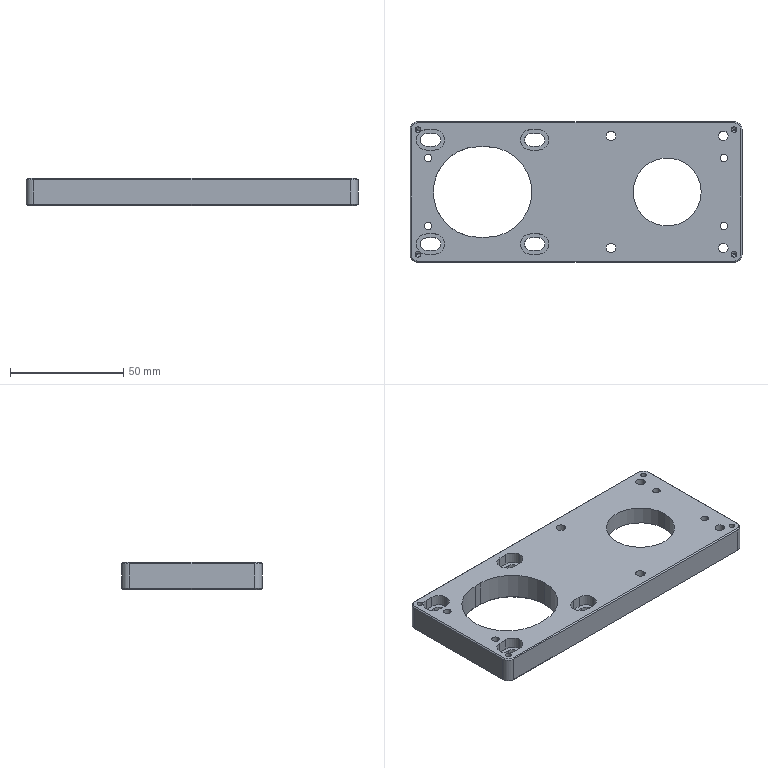Part | NX | features BREP 1 | 1 solid | 155 faces | box 146.5 x 62 x 12 mm | volume 74103 mm3 | cylinder 59 | cone 49 | plane 47 | commonest cylinder face diameters 5.5 x12 9 x12 2.5 x8 3.3 x8 4.2 x8 7 x4